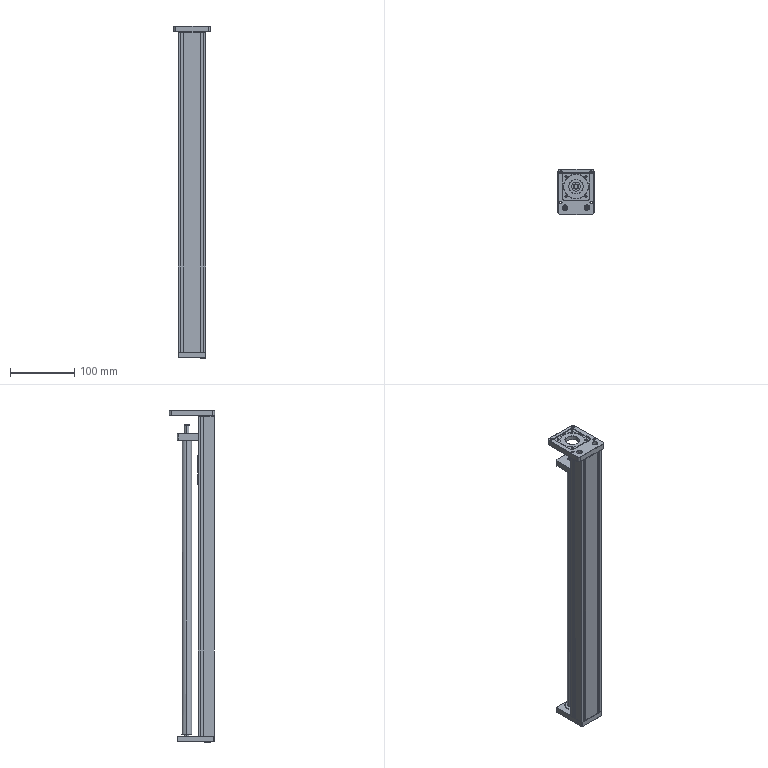Part | SolidWorks | features BaseBody 8 | 8 solids | 393 faces | box 56 x 70 x 515.8 mm | volume 426528 mm3 | plane 193 | cylinder 114 | cone 78 | torus 8 | commonest cylinder face diameters 3.3 x20 8 x16 6 x10 3 x8 3.4 x8 4.5 x8